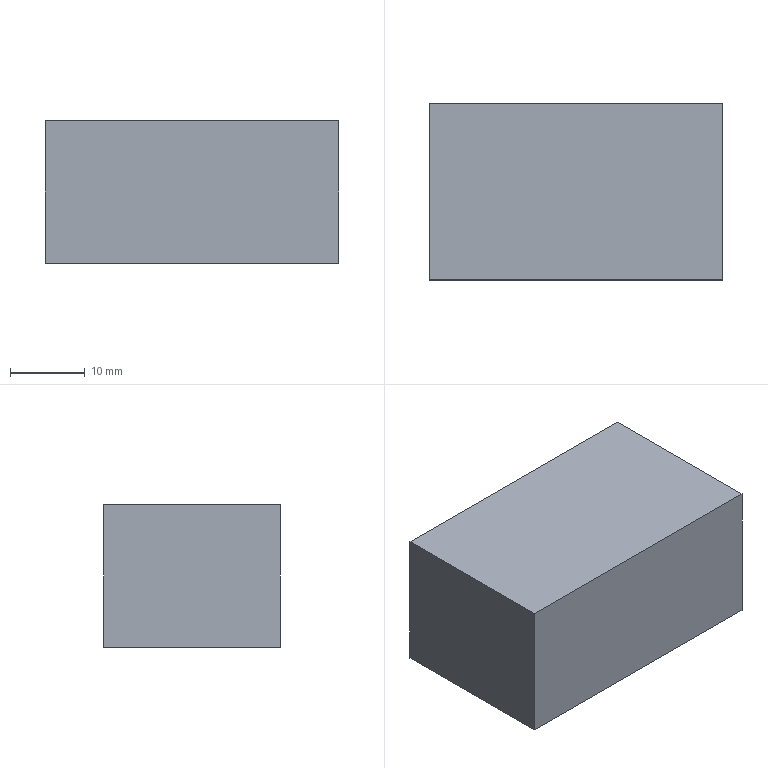Part | 1 solid | 6 faces | volume 17472 mm3 | plane 6